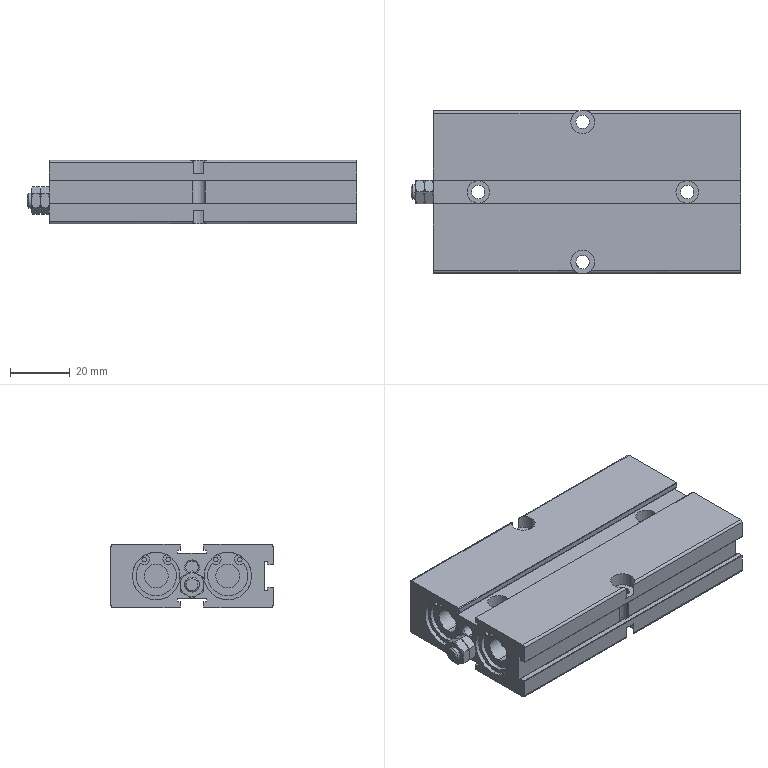Part | SolidWorks | features BaseBody 1 | 1 solid | 241 faces | box 110.5 x 54.3 x 21.2 mm | volume 77984 mm3 | cylinder 124 | plane 81 | cone 36 | commonest cylinder face diameters 0.4 x30 1.52 x16 8 x16 3.5 x12 16 x12 1.6 x8